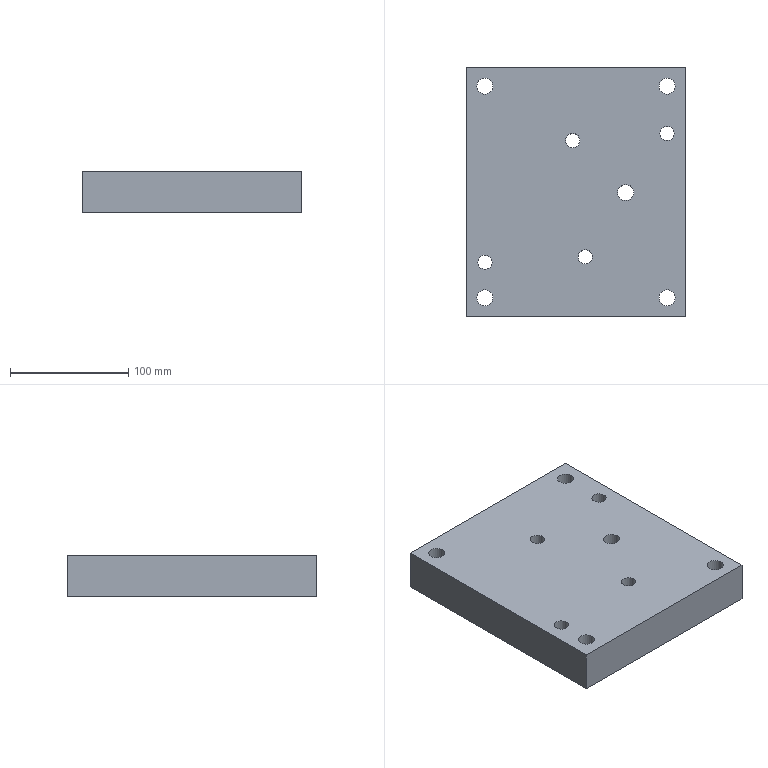Part | NX | features 7 2 | 1 solid | 37 faces | box 186 x 211 x 35 mm | volume 1310729 mm3 | cylinder 20 | plane 13 | cone 4 | commonest cylinder face diameters 13.5 x5 20 x5 10.3 x4 12.001 x4 14.11 x2
STEP:
#1=CARTESIAN_POINT('',(535.99,243.017,66.));
#2=VERTEX_POINT('',#1);
#3=CARTESIAN_POINT('',(530.84,243.017,66.));
#4=DIRECTION('',(0.,0.,1.));
#5=DIRECTION('',(1.,0.,0.));
#6=AXIS2_PLACEMENT_3D('',#3,#4,#5);
#7=CIRCLE('',#6,5.15);
#8=EDGE_CURVE('',#2,#2,#7,.T.);
#9=ORIENTED_EDGE('',*,*,#8,.T.);
#10=EDGE_LOOP('',(#9));
#11=FACE_BOUND('',#10,.T.);
#12=CARTESIAN_POINT('',(496.275,336.282,66.));
#13=VERTEX_POINT('',#12);
#14=CARTESIAN_POINT('',(490.274,336.282,66.));
#15=DIRECTION('',(0.,0.,1.));
#16=DIRECTION('',(1.,0.,0.));
#17=AXIS2_PLACEMENT_3D('',#14,#15,#16);
#18=CIRCLE('',#17,6.);
#19=EDGE_CURVE('',#13,#13,#18,.T.);
#20=ORIENTED_EDGE('',*,*,#19,.T.);
#21=EDGE_LOOP('',(#20));
#22=FACE_BOUND('',#21,.T.);
#23=CARTESIAN_POINT('',(441.424,319.282,66.));
#24=VERTEX_POINT('',#23);
#25=CARTESIAN_POINT('',(436.274,319.282,66.));
#26=DIRECTION('',(0.,0.,1.));
#27=DIRECTION('',(1.,0.,0.));
#28=AXIS2_PLACEMENT_3D('',#25,#26,#27);
#29=CIRCLE('',#28,5.15);
#30=EDGE_CURVE('',#24,#24,#29,.T.);
#31=ORIENTED_EDGE('',*,*,#30,.T.);
#32=EDGE_LOOP('',(#31));
#33=FACE_BOUND('',#32,.T.);
#34=CARTESIAN_POINT('',(577.112,342.372,66.));
#35=VERTEX_POINT('',#34);
#36=CARTESIAN_POINT('',(570.057,342.372,66.));
#37=DIRECTION('',(0.,0.,1.));
#38=DIRECTION('',(1.,0.,0.));
#39=AXIS2_PLACEMENT_3D('',#36,#37,#38);
#40=CIRCLE('',#39,7.055);
#41=EDGE_CURVE('',#35,#35,#40,.T.);
#42=ORIENTED_EDGE('',*,*,#41,.T.);
#43=EDGE_LOOP('',(#42));
#44=FACE_BOUND('',#43,.T.);
#45=CARTESIAN_POINT('',(423.112,233.372,66.));
#46=VERTEX_POINT('',#45);
#47=CARTESIAN_POINT('',(416.057,233.372,66.));
#48=DIRECTION('',(0.,0.,1.));
#49=DIRECTION('',(1.,0.,0.));
#50=AXIS2_PLACEMENT_3D('',#47,#48,#49);
#51=CIRCLE('',#50,7.055);
#52=EDGE_CURVE('',#46,#46,#51,.T.);
#53=ORIENTED_EDGE('',*,*,#52,.T.);
#54=EDGE_LOOP('',(#53));
#55=FACE_BOUND('',#54,.T.);
#56=CARTESIAN_POINT('',(525.057,292.372,66.));
#57=VERTEX_POINT('',#56);
#58=CARTESIAN_POINT('',(535.057,292.372,66.));
#59=DIRECTION('',(0.,0.,-1.));
#60=DIRECTION('',(-1.,0.,0.));
#61=AXIS2_PLACEMENT_3D('',#58,#59,#60);
#62=CIRCLE('',#61,10.);
#63=EDGE_CURVE('',#57,#57,#62,.T.);
#64=ORIENTED_EDGE('',*,*,#63,.F.);
#65=EDGE_LOOP('',(#64));
#66=FACE_BOUND('',#65,.T.);
#67=CARTESIAN_POINT('',(560.057,203.372,66.));
#68=VERTEX_POINT('',#67);
#69=CARTESIAN_POINT('',(570.057,203.372,66.));
#70=DIRECTION('',(0.,0.,1.));
#71=DIRECTION('',(-1.,0.,0.));
#72=AXIS2_PLACEMENT_3D('',#69,#70,#71);
#73=CIRCLE('',#72,10.);
#74=EDGE_CURVE('',#68,#68,#73,.T.);
#75=ORIENTED_EDGE('',*,*,#74,.T.);
#76=EDGE_LOOP('',(#75));
#77=FACE_BOUND('',#76,.T.);
#78=CARTESIAN_POINT('',(406.057,203.372,66.));
#79=VERTEX_POINT('',#78);
#80=CARTESIAN_POINT('',(416.057,203.372,66.));
#81=DIRECTION('',(0.,0.,1.));
#82=DIRECTION('',(-1.,0.,0.));
#83=AXIS2_PLACEMENT_3D('',#80,#81,#82);
#84=CIRCLE('',#83,10.);
#85=EDGE_CURVE('',#79,#79,#84,.T.);
#86=ORIENTED_EDGE('',*,*,#85,.T.);
#87=EDGE_LOOP('',(#86));
#88=FACE_BOUND('',#87,.T.);
#89=CARTESIAN_POINT('',(586.057,187.372,66.));
#90=VERTEX_POINT('',#89);
#91=CARTESIAN_POINT('',(586.057,398.372,66.));
#92=VERTEX_POINT('',#91);
#93=CARTESIAN_POINT('',(586.057,292.872,66.));
#94=DIRECTION('',(0.,1.,0.));
#95=VECTOR('',#94,1000.);
#96=LINE('',#93,#95);
#97=EDGE_CURVE('',#90,#92,#96,.T.);
#98=ORIENTED_EDGE('',*,*,#97,.F.);
#99=CARTESIAN_POINT('',(400.057,187.372,66.));
#100=VERTEX_POINT('',#99);
#101=CARTESIAN_POINT('',(493.057,187.372,66.));
#102=DIRECTION('',(1.,0.,0.));
#103=VECTOR('',#102,1000.);
#104=LINE('',#101,#103);
#105=EDGE_CURVE('',#100,#90,#104,.T.);
#106=ORIENTED_EDGE('',*,*,#105,.F.);
#107=CARTESIAN_POINT('',(400.057,398.372,66.));
#108=VERTEX_POINT('',#107);
#109=CARTESIAN_POINT('',(400.057,292.872,66.));
#110=DIRECTION('',(0.,-1.,0.));
#111=VECTOR('',#110,1000.);
#112=LINE('',#109,#111);
#113=EDGE_CURVE('',#108,#100,#112,.T.);
#114=ORIENTED_EDGE('',*,*,#113,.F.);
#115=CARTESIAN_POINT('',(493.057,398.372,66.));
#116=DIRECTION('',(-1.,0.,0.));
#117=VECTOR('',#116,1000.);
#118=LINE('',#115,#117);
#119=EDGE_CURVE('',#92,#108,#118,.T.);
#120=ORIENTED_EDGE('',*,*,#119,.F.);
#121=EDGE_LOOP('',(#98,#106,#114,#120));
#122=FACE_BOUND('',#121,.T.);
#123=CARTESIAN_POINT('',(560.057,382.372,66.));
#124=VERTEX_POINT('',#123);
#125=CARTESIAN_POINT('',(570.057,382.372,66.));
#126=DIRECTION('',(0.,0.,1.));
#127=DIRECTION('',(-1.,0.,0.));
#128=AXIS2_PLACEMENT_3D('',#125,#126,#127);
#129=CIRCLE('',#128,10.);
#130=EDGE_CURVE('',#124,#124,#129,.T.);
#131=ORIENTED_EDGE('',*,*,#130,.T.);
#132=EDGE_LOOP('',(#131));
#133=FACE_BOUND('',#132,.T.);
#134=CARTESIAN_POINT('',(406.057,382.372,66.));
#135=VERTEX_POINT('',#134);
#136=CARTESIAN_POINT('',(416.057,382.372,66.));
#137=DIRECTION('',(0.,0.,1.));
#138=DIRECTION('',(-1.,0.,0.));
#139=AXIS2_PLACEMENT_3D('',#136,#137,#138);
#140=CIRCLE('',#139,10.);
#141=EDGE_CURVE('',#135,#135,#140,.T.);
#142=ORIENTED_EDGE('',*,*,#141,.T.);
#143=EDGE_LOOP('',(#142));
#144=FACE_BOUND('',#143,.T.);
#145=CARTESIAN_POINT('',(475.99,361.282,66.));
#146=VERTEX_POINT('',#145);
#147=CARTESIAN_POINT('',(470.84,361.282,66.));
#148=DIRECTION('',(0.,0.,1.));
#149=DIRECTION('',(1.,0.,0.));
#150=AXIS2_PLACEMENT_3D('',#147,#148,#149);
#151=CIRCLE('',#150,5.15);
#152=EDGE_CURVE('',#146,#146,#151,.T.);
#153=ORIENTED_EDGE('',*,*,#152,.T.);
#154=EDGE_LOOP('',(#153));
#155=FACE_BOUND('',#154,.T.);
#156=CARTESIAN_POINT('',(506.841,238.017,66.));
#157=VERTEX_POINT('',#156);
#158=CARTESIAN_POINT('',(500.84,238.017,66.));
#159=DIRECTION('',(0.,0.,1.));
#160=DIRECTION('',(1.,0.,0.));
#161=AXIS2_PLACEMENT_3D('',#158,#159,#160);
#162=CIRCLE('',#161,6.);
#163=EDGE_CURVE('',#157,#157,#162,.T.);
#164=ORIENTED_EDGE('',*,*,#163,.T.);
#165=EDGE_LOOP('',(#164));
#166=FACE_BOUND('',#165,.T.);
#167=CARTESIAN_POINT('',(478.424,250.017,66.));
#168=VERTEX_POINT('',#167);
#169=CARTESIAN_POINT('',(473.274,250.017,66.));
#170=DIRECTION('',(0.,0.,1.));
#171=DIRECTION('',(1.,0.,0.));
#172=AXIS2_PLACEMENT_3D('',#169,#170,#171);
#173=CIRCLE('',#172,5.15);
#174=EDGE_CURVE('',#168,#168,#173,.T.);
#175=ORIENTED_EDGE('',*,*,#174,.T.);
#176=EDGE_LOOP('',(#175));
#177=FACE_BOUND('',#176,.T.);
#178=CARTESIAN_POINT('',(493.057,292.872,66.));
#179=DIRECTION('',(0.,0.,-1.));
#180=DIRECTION('',(1.,0.,0.));
#181=AXIS2_PLACEMENT_3D('',#178,#179,#180);
#182=PLANE('',#181);
#183=ADVANCED_FACE('',(#11,#22,#33,#44,#55,#66,#77,#88,#122,#133,#144,#155,#166,#177),#182,.T.);
#184=CARTESIAN_POINT('',(422.807,203.372,86.));
#185=VERTEX_POINT('',#184);
#186=CARTESIAN_POINT('',(416.057,203.372,86.));
#187=DIRECTION('',(0.,0.,1.));
#188=DIRECTION('',(1.,0.,0.));
#189=AXIS2_PLACEMENT_3D('',#186,#187,#188);
#190=CIRCLE('',#189,6.75);
#191=EDGE_CURVE('',#185,#185,#190,.T.);
#192=ORIENTED_EDGE('',*,*,#191,.T.);
#193=EDGE_LOOP('',(#192));
#194=FACE_BOUND('',#193,.T.);
#195=CARTESIAN_POINT('',(426.057,203.372,86.));
#196=VERTEX_POINT('',#195);
#197=CARTESIAN_POINT('',(416.057,203.372,86.));
#198=DIRECTION('',(0.,0.,1.));
#199=DIRECTION('',(1.,0.,0.));
#200=AXIS2_PLACEMENT_3D('',#197,#198,#199);
#201=CIRCLE('',#200,10.);
#202=EDGE_CURVE('',#196,#196,#201,.T.);
#203=ORIENTED_EDGE('',*,*,#202,.F.);
#204=EDGE_LOOP('',(#203));
#205=FACE_BOUND('',#204,.T.);
#206=CARTESIAN_POINT('',(416.057,203.372,86.));
#207=DIRECTION('',(0.,0.,1.));
#208=DIRECTION('',(-1.,0.,0.));
#209=AXIS2_PLACEMENT_3D('',#206,#207,#208);
#210=PLANE('',#209);
#211=ADVANCED_FACE('',(#194,#205),#210,.F.);
#212=CARTESIAN_POINT('',(576.807,382.372,86.));
#213=VERTEX_POINT('',#212);
#214=CARTESIAN_POINT('',(570.057,382.372,86.));
#215=DIRECTION('',(0.,0.,1.));
#216=DIRECTION('',(1.,0.,0.));
#217=AXIS2_PLACEMENT_3D('',#214,#215,#216);
#218=CIRCLE('',#217,6.75);
#219=EDGE_CURVE('',#213,#213,#218,.T.);
#220=ORIENTED_EDGE('',*,*,#219,.T.);
#221=EDGE_LOOP('',(#220));
#222=FACE_BOUND('',#221,.T.);
#223=CARTESIAN_POINT('',(580.057,382.372,86.));
#224=VERTEX_POINT('',#223);
#225=CARTESIAN_POINT('',(570.057,382.372,86.));
#226=DIRECTION('',(0.,0.,1.));
#227=DIRECTION('',(1.,0.,0.));
#228=AXIS2_PLACEMENT_3D('',#225,#226,#227);
#229=CIRCLE('',#228,10.);
#230=EDGE_CURVE('',#224,#224,#229,.T.);
#231=ORIENTED_EDGE('',*,*,#230,.F.);
#232=EDGE_LOOP('',(#231));
#233=FACE_BOUND('',#232,.T.);
#234=CARTESIAN_POINT('',(570.057,382.372,86.));
#235=DIRECTION('',(0.,0.,1.));
#236=DIRECTION('',(-1.,0.,0.));
#237=AXIS2_PLACEMENT_3D('',#234,#235,#236);
#238=PLANE('',#237);
#239=ADVANCED_FACE('',(#222,#233),#238,.F.);
#240=CARTESIAN_POINT('',(576.807,203.372,86.));
#241=VERTEX_POINT('',#240);
#242=CARTESIAN_POINT('',(570.057,203.372,86.));
#243=DIRECTION('',(0.,0.,1.));
#244=DIRECTION('',(1.,0.,0.));
#245=AXIS2_PLACEMENT_3D('',#242,#243,#244);
#246=CIRCLE('',#245,6.75);
#247=EDGE_CURVE('',#241,#241,#246,.T.);
#248=ORIENTED_EDGE('',*,*,#247,.T.);
#249=EDGE_LOOP('',(#248));
#250=FACE_BOUND('',#249,.T.);
#251=CARTESIAN_POINT('',(580.057,203.372,86.));
#252=VERTEX_POINT('',#251);
#253=CARTESIAN_POINT('',(570.057,203.372,86.));
#254=DIRECTION('',(0.,0.,1.));
#255=DIRECTION('',(1.,0.,0.));
#256=AXIS2_PLACEMENT_3D('',#253,#254,#255);
#257=CIRCLE('',#256,10.);
#258=EDGE_CURVE('',#252,#252,#257,.T.);
#259=ORIENTED_EDGE('',*,*,#258,.F.);
#260=EDGE_LOOP('',(#259));
#261=FACE_BOUND('',#260,.T.);
#262=CARTESIAN_POINT('',(570.057,203.372,86.));
#263=DIRECTION('',(0.,0.,1.));
#264=DIRECTION('',(-1.,0.,0.));
#265=AXIS2_PLACEMENT_3D('',#262,#263,#264);
#266=PLANE('',#265);
#267=ADVANCED_FACE('',(#250,#261),#266,.F.);
#268=CARTESIAN_POINT('',(422.807,382.372,86.));
#269=VERTEX_POINT('',#268);
#270=CARTESIAN_POINT('',(416.057,382.372,86.));
#271=DIRECTION('',(0.,0.,1.));
#272=DIRECTION('',(1.,0.,0.));
#273=AXIS2_PLACEMENT_3D('',#270,#271,#272);
#274=CIRCLE('',#273,6.75);
#275=EDGE_CURVE('',#269,#269,#274,.T.);
#276=ORIENTED_EDGE('',*,*,#275,.T.);
#277=EDGE_LOOP('',(#276));
#278=FACE_BOUND('',#277,.T.);
#279=CARTESIAN_POINT('',(426.057,382.372,86.));
#280=VERTEX_POINT('',#279);
#281=CARTESIAN_POINT('',(416.057,382.372,86.));
#282=DIRECTION('',(0.,0.,1.));
#283=DIRECTION('',(1.,0.,0.));
#284=AXIS2_PLACEMENT_3D('',#281,#282,#283);
#285=CIRCLE('',#284,10.);
#286=EDGE_CURVE('',#280,#280,#285,.T.);
#287=ORIENTED_EDGE('',*,*,#286,.F.);
#288=EDGE_LOOP('',(#287));
#289=FACE_BOUND('',#288,.T.);
#290=CARTESIAN_POINT('',(416.057,382.372,86.));
#291=DIRECTION('',(0.,0.,1.));
#292=DIRECTION('',(-1.,0.,0.));
#293=AXIS2_PLACEMENT_3D('',#290,#291,#292);
#294=PLANE('',#293);
#295=ADVANCED_FACE('',(#278,#289),#294,.F.);
#296=ORIENTED_EDGE('',*,*,#286,.T.);
#297=EDGE_LOOP('',(#296));
#298=FACE_BOUND('',#297,.T.);
#299=ORIENTED_EDGE('',*,*,#141,.F.);
#300=EDGE_LOOP('',(#299));
#301=FACE_BOUND('',#300,.T.);
#302=CARTESIAN_POINT('',(416.057,382.372,71.));
#303=DIRECTION('',(0.,0.,1.));
#304=DIRECTION('',(-1.,0.,0.));
#305=AXIS2_PLACEMENT_3D('',#302,#303,#304);
#306=CYLINDRICAL_SURFACE('',#305,10.);
#307=ADVANCED_FACE('',(#298,#301),#306,.F.);
#308=ORIENTED_EDGE('',*,*,#230,.T.);
#309=EDGE_LOOP('',(#308));
#310=FACE_BOUND('',#309,.T.);
#311=ORIENTED_EDGE('',*,*,#130,.F.);
#312=EDGE_LOOP('',(#311));
#313=FACE_BOUND('',#312,.T.);
#314=CARTESIAN_POINT('',(570.057,382.372,71.));
#315=DIRECTION('',(0.,0.,1.));
#316=DIRECTION('',(-1.,0.,0.));
#317=AXIS2_PLACEMENT_3D('',#314,#315,#316);
#318=CYLINDRICAL_SURFACE('',#317,10.);
#319=ADVANCED_FACE('',(#310,#313),#318,.F.);
#320=ORIENTED_EDGE('',*,*,#202,.T.);
#321=EDGE_LOOP('',(#320));
#322=FACE_BOUND('',#321,.T.);
#323=ORIENTED_EDGE('',*,*,#85,.F.);
#324=EDGE_LOOP('',(#323));
#325=FACE_BOUND('',#324,.T.);
#326=CARTESIAN_POINT('',(416.057,203.372,71.));
#327=DIRECTION('',(0.,0.,1.));
#328=DIRECTION('',(-1.,0.,0.));
#329=AXIS2_PLACEMENT_3D('',#326,#327,#328);
#330=CYLINDRICAL_SURFACE('',#329,10.);
#331=ADVANCED_FACE('',(#322,#325),#330,.F.);
#332=ORIENTED_EDGE('',*,*,#258,.T.);
#333=EDGE_LOOP('',(#332));
#334=FACE_BOUND('',#333,.T.);
#335=ORIENTED_EDGE('',*,*,#74,.F.);
#336=EDGE_LOOP('',(#335));
#337=FACE_BOUND('',#336,.T.);
#338=CARTESIAN_POINT('',(570.057,203.372,71.));
#339=DIRECTION('',(0.,0.,1.));
#340=DIRECTION('',(-1.,0.,0.));
#341=AXIS2_PLACEMENT_3D('',#338,#339,#340);
#342=CYLINDRICAL_SURFACE('',#341,10.);
#343=ADVANCED_FACE('',(#334,#337),#342,.F.);
#344=CARTESIAN_POINT('',(400.057,187.372,101.));
#345=VERTEX_POINT('',#344);
#346=CARTESIAN_POINT('',(400.057,187.372,71.));
#347=DIRECTION('',(0.,0.,1.));
#348=VECTOR('',#347,1000.);
#349=LINE('',#346,#348);
#350=EDGE_CURVE('',#100,#345,#349,.T.);
#351=ORIENTED_EDGE('',*,*,#350,.T.);
#352=CARTESIAN_POINT('',(400.057,398.372,101.));
#353=VERTEX_POINT('',#352);
#354=CARTESIAN_POINT('',(400.057,292.872,101.));
#355=DIRECTION('',(0.,1.,0.));
#356=VECTOR('',#355,1000.);
#357=LINE('',#354,#356);
#358=EDGE_CURVE('',#345,#353,#357,.T.);
#359=ORIENTED_EDGE('',*,*,#358,.T.);
#360=CARTESIAN_POINT('',(400.057,398.372,71.));
#361=DIRECTION('',(0.,0.,1.));
#362=VECTOR('',#361,1000.);
#363=LINE('',#360,#362);
#364=EDGE_CURVE('',#108,#353,#363,.T.);
#365=ORIENTED_EDGE('',*,*,#364,.F.);
#366=ORIENTED_EDGE('',*,*,#113,.T.);
#367=EDGE_LOOP('',(#351,#359,#365,#366));
#368=FACE_BOUND('',#367,.T.);
#369=CARTESIAN_POINT('',(400.057,292.872,71.));
#370=DIRECTION('',(-1.,0.,0.));
#371=DIRECTION('',(0.,0.,-1.));
#372=AXIS2_PLACEMENT_3D('',#369,#370,#371);
#373=PLANE('',#372);
#374=ADVANCED_FACE('',(#368),#373,.T.);
#375=ORIENTED_EDGE('',*,*,#364,.T.);
#376=CARTESIAN_POINT('',(586.057,398.372,101.));
#377=VERTEX_POINT('',#376);
#378=CARTESIAN_POINT('',(493.057,398.372,101.));
#379=DIRECTION('',(1.,0.,0.));
#380=VECTOR('',#379,1000.);
#381=LINE('',#378,#380);
#382=EDGE_CURVE('',#353,#377,#381,.T.);
#383=ORIENTED_EDGE('',*,*,#382,.T.);
#384=CARTESIAN_POINT('',(586.057,398.372,71.));
#385=DIRECTION('',(0.,0.,1.));
#386=VECTOR('',#385,1000.);
#387=LINE('',#384,#386);
#388=EDGE_CURVE('',#92,#377,#387,.T.);
#389=ORIENTED_EDGE('',*,*,#388,.F.);
#390=ORIENTED_EDGE('',*,*,#119,.T.);
#391=EDGE_LOOP('',(#375,#383,#389,#390));
#392=FACE_BOUND('',#391,.T.);
#393=CARTESIAN_POINT('',(493.057,398.372,71.));
#394=DIRECTION('',(0.,1.,0.));
#395=DIRECTION('',(0.,0.,-1.));
#396=AXIS2_PLACEMENT_3D('',#393,#394,#395);
#397=PLANE('',#396);
#398=ADVANCED_FACE('',(#392),#397,.T.);
#399=ORIENTED_EDGE('',*,*,#97,.T.);
#400=ORIENTED_EDGE('',*,*,#388,.T.);
#401=CARTESIAN_POINT('',(586.057,187.372,101.));
#402=VERTEX_POINT('',#401);
#403=CARTESIAN_POINT('',(586.057,292.872,101.));
#404=DIRECTION('',(0.,-1.,0.));
#405=VECTOR('',#404,1000.);
#406=LINE('',#403,#405);
#407=EDGE_CURVE('',#377,#402,#406,.T.);
#408=ORIENTED_EDGE('',*,*,#407,.T.);
#409=CARTESIAN_POINT('',(586.057,187.372,71.));
#410=DIRECTION('',(0.,0.,1.));
#411=VECTOR('',#410,1000.);
#412=LINE('',#409,#411);
#413=EDGE_CURVE('',#90,#402,#412,.T.);
#414=ORIENTED_EDGE('',*,*,#413,.F.);
#415=EDGE_LOOP('',(#399,#400,#408,#414));
#416=FACE_BOUND('',#415,.T.);
#417=CARTESIAN_POINT('',(586.057,292.872,71.));
#418=DIRECTION('',(1.,0.,0.));
#419=DIRECTION('',(0.,0.,1.));
#420=AXIS2_PLACEMENT_3D('',#417,#418,#419);
#421=PLANE('',#420);
#422=ADVANCED_FACE('',(#416),#421,.T.);
#423=ORIENTED_EDGE('',*,*,#413,.T.);
#424=CARTESIAN_POINT('',(493.057,187.372,101.));
#425=DIRECTION('',(-1.,0.,0.));
#426=VECTOR('',#425,1000.);
#427=LINE('',#424,#426);
#428=EDGE_CURVE('',#402,#345,#427,.T.);
#429=ORIENTED_EDGE('',*,*,#428,.T.);
#430=ORIENTED_EDGE('',*,*,#350,.F.);
#431=ORIENTED_EDGE('',*,*,#105,.T.);
#432=EDGE_LOOP('',(#423,#429,#430,#431));
#433=FACE_BOUND('',#432,.T.);
#434=CARTESIAN_POINT('',(493.057,187.372,71.));
#435=DIRECTION('',(0.,-1.,0.));
#436=DIRECTION('',(0.,0.,1.));
#437=AXIS2_PLACEMENT_3D('',#434,#435,#436);
#438=PLANE('',#437);
#439=ADVANCED_FACE('',(#433),#438,.T.);
#440=CARTESIAN_POINT('',(422.807,203.372,101.));
#441=VERTEX_POINT('',#440);
#442=CARTESIAN_POINT('',(416.057,203.372,101.));
#443=DIRECTION('',(0.,0.,1.));
#444=DIRECTION('',(1.,0.,0.));
#445=AXIS2_PLACEMENT_3D('',#442,#443,#444);
#446=CIRCLE('',#445,6.75);
#447=EDGE_CURVE('',#441,#441,#446,.T.);
#448=ORIENTED_EDGE('',*,*,#447,.T.);
#449=EDGE_LOOP('',(#448));
#450=FACE_BOUND('',#449,.T.);
#451=ORIENTED_EDGE('',*,*,#191,.F.);
#452=EDGE_LOOP('',(#451));
#453=FACE_BOUND('',#452,.T.);
#454=CARTESIAN_POINT('',(416.057,203.372,68.));
#455=DIRECTION('',(0.,0.,1.));
#456=DIRECTION('',(-1.,0.,0.));
#457=AXIS2_PLACEMENT_3D('',#454,#455,#456);
#458=CYLINDRICAL_SURFACE('',#457,6.75);
#459=ADVANCED_FACE('',(#450,#453),#458,.F.);
#460=CARTESIAN_POINT('',(576.807,382.372,101.));
#461=VERTEX_POINT('',#460);
#462=CARTESIAN_POINT('',(570.057,382.372,101.));
#463=DIRECTION('',(0.,0.,1.));
#464=DIRECTION('',(1.,0.,0.));
#465=AXIS2_PLACEMENT_3D('',#462,#463,#464);
#466=CIRCLE('',#465,6.75);
#467=EDGE_CURVE('',#461,#461,#466,.T.);
#468=ORIENTED_EDGE('',*,*,#467,.T.);
#469=EDGE_LOOP('',(#468));
#470=FACE_BOUND('',#469,.T.);
#471=ORIENTED_EDGE('',*,*,#219,.F.);
#472=EDGE_LOOP('',(#471));
#473=FACE_BOUND('',#472,.T.);
#474=CARTESIAN_POINT('',(570.057,382.372,68.));
#475=DIRECTION('',(0.,0.,1.));
#476=DIRECTION('',(-1.,0.,0.));
#477=AXIS2_PLACEMENT_3D('',#474,#475,#476);
#478=CYLINDRICAL_SURFACE('',#477,6.75);
#479=ADVANCED_FACE('',(#470,#473),#478,.F.);
#480=CARTESIAN_POINT('',(576.807,203.372,101.));
#481=VERTEX_POINT('',#480);
#482=CARTESIAN_POINT('',(570.057,203.372,101.));
#483=DIRECTION('',(0.,0.,1.));
#484=DIRECTION('',(1.,0.,0.));
#485=AXIS2_PLACEMENT_3D('',#482,#483,#484);
#486=CIRCLE('',#485,6.75);
#487=EDGE_CURVE('',#481,#481,#486,.T.);
#488=ORIENTED_EDGE('',*,*,#487,.T.);
#489=EDGE_LOOP('',(#488));
#490=FACE_BOUND('',#489,.T.);
#491=ORIENTED_EDGE('',*,*,#247,.F.);
#492=EDGE_LOOP('',(#491));
#493=FACE_BOUND('',#492,.T.);
#494=CARTESIAN_POINT('',(570.057,203.372,68.));
#495=DIRECTION('',(0.,0.,1.));
#496=DIRECTION('',(-1.,0.,0.));
#497=AXIS2_PLACEMENT_3D('',#494,#495,#496);
#498=CYLINDRICAL_SURFACE('',#497,6.75);
#499=ADVANCED_FACE('',(#490,#493),#498,.F.);
#500=CARTESIAN_POINT('',(422.807,382.372,101.));
#501=VERTEX_POINT('',#500);
#502=CARTESIAN_POINT('',(416.057,382.372,101.));
#503=DIRECTION('',(0.,0.,1.));
#504=DIRECTION('',(1.,0.,0.));
#505=AXIS2_PLACEMENT_3D('',#502,#503,#504);
#506=CIRCLE('',#505,6.75);
#507=EDGE_CURVE('',#501,#501,#506,.T.);
#508=ORIENTED_EDGE('',*,*,#507,.T.);
#509=EDGE_LOOP('',(#508));
#510=FACE_BOUND('',#509,.T.);
#511=ORIENTED_EDGE('',*,*,#275,.F.);
#512=EDGE_LOOP('',(#511));
#513=FACE_BOUND('',#512,.T.);
#514=CARTESIAN_POINT('',(416.057,382.372,68.));
#515=DIRECTION('',(0.,0.,1.));
#516=DIRECTION('',(-1.,0.,0.));
#517=AXIS2_PLACEMENT_3D('',#514,#515,#516);
#518=CYLINDRICAL_SURFACE('',#517,6.75);
#519=ADVANCED_FACE('',(#510,#513),#518,.F.);
#520=CARTESIAN_POINT('',(422.058,233.372,78.));
#521=VERTEX_POINT('',#520);
#522=CARTESIAN_POINT('',(416.057,233.372,78.));
#523=DIRECTION('',(0.,0.,-1.));
#524=DIRECTION('',(1.,0.,0.));
#525=AXIS2_PLACEMENT_3D('',#522,#523,#524);
#526=CIRCLE('',#525,6.);
#527=EDGE_CURVE('',#521,#521,#526,.T.);
#528=ORIENTED_EDGE('',*,*,#527,.T.);
#529=EDGE_LOOP('',(#528));
#530=FACE_BOUND('',#529,.T.);
#531=CARTESIAN_POINT('',(422.058,233.372,101.));
#532=VERTEX_POINT('',#531);
#533=CARTESIAN_POINT('',(416.057,233.372,101.));
#534=DIRECTION('',(0.,0.,1.));
#535=DIRECTION('',(1.,0.,0.));
#536=AXIS2_PLACEMENT_3D('',#533,#534,#535);
#537=CIRCLE('',#536,6.);
#538=EDGE_CURVE('',#532,#532,#537,.T.);
#539=ORIENTED_EDGE('',*,*,#538,.T.);
#540=EDGE_LOOP('',(#539));
#541=FACE_BOUND('',#540,.T.);
#542=CARTESIAN_POINT('',(416.057,233.372,68.));
#543=DIRECTION('',(0.,0.,1.));
#544=DIRECTION('',(-1.,0.,0.));
#545=AXIS2_PLACEMENT_3D('',#542,#543,#544);
#546=CYLINDRICAL_SURFACE('',#545,6.);
#547=ADVANCED_FACE('',(#530,#541),#546,.F.);
#548=CARTESIAN_POINT('',(576.058,342.372,78.));
#549=VERTEX_POINT('',#548);
#550=CARTESIAN_POINT('',(570.057,342.372,78.));
#551=DIRECTION('',(0.,0.,-1.));
#552=DIRECTION('',(1.,0.,0.));
#553=AXIS2_PLACEMENT_3D('',#550,#551,#552);
#554=CIRCLE('',#553,6.);
#555=EDGE_CURVE('',#549,#549,#554,.T.);
#556=ORIENTED_EDGE('',*,*,#555,.T.);
#557=EDGE_LOOP('',(#556));
#558=FACE_BOUND('',#557,.T.);
#559=CARTESIAN_POINT('',(576.058,342.372,101.));
#560=VERTEX_POINT('',#559);
#561=CARTESIAN_POINT('',(570.057,342.372,101.));
#562=DIRECTION('',(0.,0.,1.));
#563=DIRECTION('',(1.,0.,0.));
#564=AXIS2_PLACEMENT_3D('',#561,#562,#563);
#565=CIRCLE('',#564,6.);
#566=EDGE_CURVE('',#560,#560,#565,.T.);
#567=ORIENTED_EDGE('',*,*,#566,.T.);
#568=EDGE_LOOP('',(#567));
#569=FACE_BOUND('',#568,.T.);
#570=CARTESIAN_POINT('',(570.057,342.372,68.));
#571=DIRECTION('',(0.,0.,1.));
#572=DIRECTION('',(-1.,0.,0.));
#573=AXIS2_PLACEMENT_3D('',#570,#571,#572);
#574=CYLINDRICAL_SURFACE('',#573,6.);
#575=ADVANCED_FACE('',(#558,#569),#574,.F.);
#576=CARTESIAN_POINT('',(506.841,238.017,101.));
#577=VERTEX_POINT('',#576);
#578=CARTESIAN_POINT('',(500.84,238.017,101.));
#579=DIRECTION('',(0.,0.,1.));
#580=DIRECTION('',(1.,0.,0.));
#581=AXIS2_PLACEMENT_3D('',#578,#579,#580);
#582=CIRCLE('',#581,6.);
#583=EDGE_CURVE('',#577,#577,#582,.T.);
#584=ORIENTED_EDGE('',*,*,#583,.F.);
#585=EDGE_LOOP('',(#584));
#586=FACE_BOUND('',#585,.T.);
#587=CARTESIAN_POINT('',(496.275,336.282,101.));
#588=VERTEX_POINT('',#587);
#589=CARTESIAN_POINT('',(490.274,336.282,101.));
#590=DIRECTION('',(0.,0.,1.));
#591=DIRECTION('',(1.,0.,0.));
#592=AXIS2_PLACEMENT_3D('',#589,#590,#591);
#593=CIRCLE('',#592,6.);
#594=EDGE_CURVE('',#588,#588,#593,.T.);
#595=ORIENTED_EDGE('',*,*,#594,.F.);
#596=EDGE_LOOP('',(#595));
#597=FACE_BOUND('',#596,.T.);
#598=CARTESIAN_POINT('',(541.807,292.372,101.));
#599=VERTEX_POINT('',#598);
#600=CARTESIAN_POINT('',(535.057,292.372,101.));
#601=DIRECTION('',(0.,0.,1.));
#602=DIRECTION('',(1.,0.,0.));
#603=AXIS2_PLACEMENT_3D('',#600,#601,#602);
#604=CIRCLE('',#603,6.75);
#605=EDGE_CURVE('',#599,#599,#604,.T.);
#606=ORIENTED_EDGE('',*,*,#605,.F.);
#607=EDGE_LOOP('',(#606));
#608=FACE_BOUND('',#607,.T.);
#609=ORIENTED_EDGE('',*,*,#566,.F.);
#610=EDGE_LOOP('',(#609));
#611=FACE_BOUND('',#610,.T.);
#612=ORIENTED_EDGE('',*,*,#538,.F.);
#613=EDGE_LOOP('',(#612));
#614=FACE_BOUND('',#613,.T.);
#615=ORIENTED_EDGE('',*,*,#507,.F.);
#616=EDGE_LOOP('',(#615));
#617=FACE_BOUND('',#616,.T.);
#618=ORIENTED_EDGE('',*,*,#487,.F.);
#619=EDGE_LOOP('',(#618));
#620=FACE_BOUND('',#619,.T.);
#621=ORIENTED_EDGE('',*,*,#467,.F.);
#622=EDGE_LOOP('',(#621));
#623=FACE_BOUND('',#622,.T.);
#624=ORIENTED_EDGE('',*,*,#447,.F.);
#625=EDGE_LOOP('',(#624));
#626=FACE_BOUND('',#625,.T.);
#627=ORIENTED_EDGE('',*,*,#428,.F.);
#628=ORIENTED_EDGE('',*,*,#407,.F.);
#629=ORIENTED_EDGE('',*,*,#382,.F.);
#630=ORIENTED_EDGE('',*,*,#358,.F.);
#631=EDGE_LOOP('',(#627,#628,#629,#630));
#632=FACE_BOUND('',#631,.T.);
#633=CARTESIAN_POINT('',(493.057,292.872,101.));
#634=DIRECTION('',(0.,0.,1.));
#635=DIRECTION('',(-1.,0.,0.));
#636=AXIS2_PLACEMENT_3D('',#633,#634,#635);
#637=PLANE('',#636);
#638=ADVANCED_FACE('',(#586,#597,#608,#611,#614,#617,#620,#623,#626,#632),#637,.T.);
#639=CARTESIAN_POINT('',(541.807,292.372,86.));
#640=VERTEX_POINT('',#639);
#641=CARTESIAN_POINT('',(535.057,292.372,86.));
#642=DIRECTION('',(0.,0.,1.));
#643=DIRECTION('',(1.,0.,0.));
#644=AXIS2_PLACEMENT_3D('',#641,#642,#643);
#645=CIRCLE('',#644,6.75);
#646=EDGE_CURVE('',#640,#640,#645,.T.);
#647=ORIENTED_EDGE('',*,*,#646,.T.);
#648=EDGE_LOOP('',(#647));
#649=FACE_BOUND('',#648,.T.);
#650=CARTESIAN_POINT('',(545.057,292.372,86.));
#651=VERTEX_POINT('',#650);
#652=CARTESIAN_POINT('',(535.057,292.372,86.));
#653=DIRECTION('',(0.,0.,1.));
#654=DIRECTION('',(1.,0.,0.));
#655=AXIS2_PLACEMENT_3D('',#652,#653,#654);
#656=CIRCLE('',#655,10.);
#657=EDGE_CURVE('',#651,#651,#656,.T.);
#658=ORIENTED_EDGE('',*,*,#657,.F.);
#659=EDGE_LOOP('',(#658));
#660=FACE_BOUND('',#659,.T.);
#661=CARTESIAN_POINT('',(535.057,292.372,86.));
#662=DIRECTION('',(0.,0.,1.));
#663=DIRECTION('',(-1.,0.,0.));
#664=AXIS2_PLACEMENT_3D('',#661,#662,#663);
#665=PLANE('',#664);
#666=ADVANCED_FACE('',(#649,#660),#665,.F.);
#667=ORIENTED_EDGE('',*,*,#605,.T.);
#668=EDGE_LOOP('',(#667));
#669=FACE_BOUND('',#668,.T.);
#670=ORIENTED_EDGE('',*,*,#646,.F.);
#671=EDGE_LOOP('',(#670));
#672=FACE_BOUND('',#671,.T.);
#673=CARTESIAN_POINT('',(535.057,292.372,68.));
#674=DIRECTION('',(0.,0.,1.));
#675=DIRECTION('',(-1.,0.,0.));
#676=AXIS2_PLACEMENT_3D('',#673,#674,#675);
#677=CYLINDRICAL_SURFACE('',#676,6.75);
#678=ADVANCED_FACE('',(#669,#672),#677,.F.);
#679=ORIENTED_EDGE('',*,*,#657,.T.);
#680=EDGE_LOOP('',(#679));
#681=FACE_BOUND('',#680,.T.);
#682=ORIENTED_EDGE('',*,*,#63,.T.);
#683=EDGE_LOOP('',(#682));
#684=FACE_BOUND('',#683,.T.);
#685=CARTESIAN_POINT('',(535.057,292.372,71.));
#686=DIRECTION('',(0.,0.,1.));
#687=DIRECTION('',(-1.,0.,0.));
#688=AXIS2_PLACEMENT_3D('',#685,#686,#687);
#689=CYLINDRICAL_SURFACE('',#688,10.);
#690=ADVANCED_FACE('',(#681,#684),#689,.F.);
#691=CARTESIAN_POINT('',(423.112,233.372,78.));
#692=VERTEX_POINT('',#691);
#693=CARTESIAN_POINT('',(416.057,233.372,78.));
#694=DIRECTION('',(0.,0.,-1.));
#695=DIRECTION('',(1.,0.,0.));
#696=AXIS2_PLACEMENT_3D('',#693,#694,#695);
#697=CIRCLE('',#696,7.055);
#698=EDGE_CURVE('',#692,#692,#697,.T.);
#699=ORIENTED_EDGE('',*,*,#698,.T.);
#700=EDGE_LOOP('',(#699));
#701=FACE_BOUND('',#700,.T.);
#702=ORIENTED_EDGE('',*,*,#527,.F.);
#703=EDGE_LOOP('',(#702));
#704=FACE_BOUND('',#703,.T.);
#705=CARTESIAN_POINT('',(416.057,233.372,78.));
#706=DIRECTION('',(0.,0.,1.));
#707=DIRECTION('',(-1.,0.,0.));
#708=AXIS2_PLACEMENT_3D('',#705,#706,#707);
#709=PLANE('',#708);
#710=ADVANCED_FACE('',(#701,#704),#709,.F.);
#711=ORIENTED_EDGE('',*,*,#698,.F.);
#712=EDGE_LOOP('',(#711));
#713=FACE_BOUND('',#712,.T.);
#714=ORIENTED_EDGE('',*,*,#52,.F.);
#715=EDGE_LOOP('',(#714));
#716=FACE_BOUND('',#715,.T.);
#717=CARTESIAN_POINT('',(416.057,233.372,66.));
#718=DIRECTION('',(0.,0.,1.));
#719=DIRECTION('',(-1.,0.,0.));
#720=AXIS2_PLACEMENT_3D('',#717,#718,#719);
#721=CYLINDRICAL_SURFACE('',#720,7.055);
#722=ADVANCED_FACE('',(#713,#716),#721,.F.);
#723=CARTESIAN_POINT('',(577.112,342.372,78.));
#724=VERTEX_POINT('',#723);
#725=CARTESIAN_POINT('',(570.057,342.372,78.));
#726=DIRECTION('',(0.,0.,-1.));
#727=DIRECTION('',(1.,0.,0.));
#728=AXIS2_PLACEMENT_3D('',#725,#726,#727);
#729=CIRCLE('',#728,7.055);
#730=EDGE_CURVE('',#724,#724,#729,.T.);
#731=ORIENTED_EDGE('',*,*,#730,.T.);
#732=EDGE_LOOP('',(#731));
#733=FACE_BOUND('',#732,.T.);
#734=ORIENTED_EDGE('',*,*,#555,.F.);
#735=EDGE_LOOP('',(#734));
#736=FACE_BOUND('',#735,.T.);
#737=CARTESIAN_POINT('',(570.057,342.372,78.));
#738=DIRECTION('',(0.,0.,1.));
#739=DIRECTION('',(-1.,0.,0.));
#740=AXIS2_PLACEMENT_3D('',#737,#738,#739);
#741=PLANE('',#740);
#742=ADVANCED_FACE('',(#733,#736),#741,.F.);
#743=ORIENTED_EDGE('',*,*,#730,.F.);
#744=EDGE_LOOP('',(#743));
#745=FACE_BOUND('',#744,.T.);
#746=ORIENTED_EDGE('',*,*,#41,.F.);
#747=EDGE_LOOP('',(#746));
#748=FACE_BOUND('',#747,.T.);
#749=CARTESIAN_POINT('',(570.057,342.372,66.));
#750=DIRECTION('',(0.,0.,1.));
#751=DIRECTION('',(-1.,0.,0.));
#752=AXIS2_PLACEMENT_3D('',#749,#750,#751);
#753=CYLINDRICAL_SURFACE('',#752,7.055);
#754=ADVANCED_FACE('',(#745,#748),#753,.F.);
#755=CARTESIAN_POINT('',(441.424,319.282,75.85));
#756=VERTEX_POINT('',#755);
#757=CARTESIAN_POINT('',(436.274,319.282,75.85));
#758=DIRECTION('',(0.,0.,1.));
#759=DIRECTION('',(1.,0.,0.));
#760=AXIS2_PLACEMENT_3D('',#757,#758,#759);
#761=CIRCLE('',#760,5.15);
#762=EDGE_CURVE('',#756,#756,#761,.T.);
#763=ORIENTED_EDGE('',*,*,#762,.T.);
#764=EDGE_LOOP('',(#763));
#765=FACE_BOUND('',#764,.T.);
#766=ORIENTED_EDGE('',*,*,#30,.F.);
#767=EDGE_LOOP('',(#766));
#768=FACE_BOUND('',#767,.T.);
#769=CARTESIAN_POINT('',(436.274,319.282,66.));
#770=DIRECTION('',(0.,0.,1.));
#771=DIRECTION('',(-1.,0.,0.));
#772=AXIS2_PLACEMENT_3D('',#769,#770,#771);
#773=CYLINDRICAL_SURFACE('',#772,5.15);
#774=ADVANCED_FACE('',(#765,#768),#773,.F.);
#775=CARTESIAN_POINT('',(436.274,319.282,81.));
#776=VERTEX_POINT('',#775);
#777=VERTEX_LOOP('',#776);
#778=FACE_BOUND('',#777,.T.);
#779=ORIENTED_EDGE('',*,*,#762,.F.);
#780=EDGE_LOOP('',(#779));
#781=FACE_BOUND('',#780,.T.);
#782=CARTESIAN_POINT('',(436.274,319.282,75.85));
#783=DIRECTION('',(0.,0.,-1.));
#784=DIRECTION('',(1.,0.,0.));
#785=AXIS2_PLACEMENT_3D('',#782,#783,#784);
#786=CONICAL_SURFACE('',#785,5.15,0.7854);
#787=ADVANCED_FACE('',(#778,#781),#786,.F.);
#788=CARTESIAN_POINT('',(475.99,361.282,75.85));
#789=VERTEX_POINT('',#788);
#790=CARTESIAN_POINT('',(470.84,361.282,75.85));
#791=DIRECTION('',(0.,0.,1.));
#792=DIRECTION('',(1.,0.,0.));
#793=AXIS2_PLACEMENT_3D('',#790,#791,#792);
#794=CIRCLE('',#793,5.15);
#795=EDGE_CURVE('',#789,#789,#794,.T.);
#796=ORIENTED_EDGE('',*,*,#795,.T.);
#797=EDGE_LOOP('',(#796));
#798=FACE_BOUND('',#797,.T.);
#799=ORIENTED_EDGE('',*,*,#152,.F.);
#800=EDGE_LOOP('',(#799));
#801=FACE_BOUND('',#800,.T.);
#802=CARTESIAN_POINT('',(470.84,361.282,66.));
#803=DIRECTION('',(0.,0.,1.));
#804=DIRECTION('',(-1.,0.,0.));
#805=AXIS2_PLACEMENT_3D('',#802,#803,#804);
#806=CYLINDRICAL_SURFACE('',#805,5.15);
#807=ADVANCED_FACE('',(#798,#801),#806,.F.);
#808=CARTESIAN_POINT('',(470.84,361.282,81.));
#809=VERTEX_POINT('',#808);
#810=VERTEX_LOOP('',#809);
#811=FACE_BOUND('',#810,.T.);
#812=ORIENTED_EDGE('',*,*,#795,.F.);
#813=EDGE_LOOP('',(#812));
#814=FACE_BOUND('',#813,.T.);
#815=CARTESIAN_POINT('',(470.84,361.282,75.85));
#816=DIRECTION('',(0.,0.,-1.));
#817=DIRECTION('',(1.,0.,0.));
#818=AXIS2_PLACEMENT_3D('',#815,#816,#817);
#819=CONICAL_SURFACE('',#818,5.15,0.7854);
#820=ADVANCED_FACE('',(#811,#814),#819,.F.);
#821=ORIENTED_EDGE('',*,*,#594,.T.);
#822=EDGE_LOOP('',(#821));
#823=FACE_BOUND('',#822,.T.);
#824=ORIENTED_EDGE('',*,*,#19,.F.);
#825=EDGE_LOOP('',(#824));
#826=FACE_BOUND('',#825,.T.);
#827=CARTESIAN_POINT('',(490.274,336.282,66.));
#828=DIRECTION('',(0.,0.,1.));
#829=DIRECTION('',(-1.,0.,0.));
#830=AXIS2_PLACEMENT_3D('',#827,#828,#829);
#831=CYLINDRICAL_SURFACE('',#830,6.);
#832=ADVANCED_FACE('',(#823,#826),#831,.F.);
#833=ORIENTED_EDGE('',*,*,#583,.T.);
#834=EDGE_LOOP('',(#833));
#835=FACE_BOUND('',#834,.T.);
#836=ORIENTED_EDGE('',*,*,#163,.F.);
#837=EDGE_LOOP('',(#836));
#838=FACE_BOUND('',#837,.T.);
#839=CARTESIAN_POINT('',(500.84,238.017,66.));
#840=DIRECTION('',(0.,0.,1.));
#841=DIRECTION('',(-1.,0.,0.));
#842=AXIS2_PLACEMENT_3D('',#839,#840,#841);
#843=CYLINDRICAL_SURFACE('',#842,6.);
#844=ADVANCED_FACE('',(#835,#838),#843,.F.);
#845=CARTESIAN_POINT('',(535.99,243.017,75.85));
#846=VERTEX_POINT('',#845);
#847=CARTESIAN_POINT('',(530.84,243.017,75.85));
#848=DIRECTION('',(0.,0.,1.));
#849=DIRECTION('',(1.,0.,0.));
#850=AXIS2_PLACEMENT_3D('',#847,#848,#849);
#851=CIRCLE('',#850,5.15);
#852=EDGE_CURVE('',#846,#846,#851,.T.);
#853=ORIENTED_EDGE('',*,*,#852,.T.);
#854=EDGE_LOOP('',(#853));
#855=FACE_BOUND('',#854,.T.);
#856=ORIENTED_EDGE('',*,*,#8,.F.);
#857=EDGE_LOOP('',(#856));
#858=FACE_BOUND('',#857,.T.);
#859=CARTESIAN_POINT('',(530.84,243.017,66.));
#860=DIRECTION('',(0.,0.,1.));
#861=DIRECTION('',(-1.,0.,0.));
#862=AXIS2_PLACEMENT_3D('',#859,#860,#861);
#863=CYLINDRICAL_SURFACE('',#862,5.15);
#864=ADVANCED_FACE('',(#855,#858),#863,.F.);
#865=CARTESIAN_POINT('',(530.84,243.017,81.));
#866=VERTEX_POINT('',#865);
#867=VERTEX_LOOP('',#866);
#868=FACE_BOUND('',#867,.T.);
#869=ORIENTED_EDGE('',*,*,#852,.F.);
#870=EDGE_LOOP('',(#869));
#871=FACE_BOUND('',#870,.T.);
#872=CARTESIAN_POINT('',(530.84,243.017,75.85));
#873=DIRECTION('',(0.,0.,-1.));
#874=DIRECTION('',(1.,0.,0.));
#875=AXIS2_PLACEMENT_3D('',#872,#873,#874);
#876=CONICAL_SURFACE('',#875,5.15,0.7854);
#877=ADVANCED_FACE('',(#868,#871),#876,.F.);
#878=CARTESIAN_POINT('',(478.424,250.017,75.85));
#879=VERTEX_POINT('',#878);
#880=CARTESIAN_POINT('',(473.274,250.017,75.85));
#881=DIRECTION('',(0.,0.,1.));
#882=DIRECTION('',(1.,0.,0.));
#883=AXIS2_PLACEMENT_3D('',#880,#881,#882);
#884=CIRCLE('',#883,5.15);
#885=EDGE_CURVE('',#879,#879,#884,.T.);
#886=ORIENTED_EDGE('',*,*,#885,.T.);
#887=EDGE_LOOP('',(#886));
#888=FACE_BOUND('',#887,.T.);
#889=ORIENTED_EDGE('',*,*,#174,.F.);
#890=EDGE_LOOP('',(#889));
#891=FACE_BOUND('',#890,.T.);
#892=CARTESIAN_POINT('',(473.274,250.017,66.));
#893=DIRECTION('',(0.,0.,1.));
#894=DIRECTION('',(-1.,0.,0.));
#895=AXIS2_PLACEMENT_3D('',#892,#893,#894);
#896=CYLINDRICAL_SURFACE('',#895,5.15);
#897=ADVANCED_FACE('',(#888,#891),#896,.F.);
#898=CARTESIAN_POINT('',(473.274,250.017,81.));
#899=VERTEX_POINT('',#898);
#900=VERTEX_LOOP('',#899);
#901=FACE_BOUND('',#900,.T.);
#902=ORIENTED_EDGE('',*,*,#885,.F.);
#903=EDGE_LOOP('',(#902));
#904=FACE_BOUND('',#903,.T.);
#905=CARTESIAN_POINT('',(473.274,250.017,75.85));
#906=DIRECTION('',(0.,0.,-1.));
#907=DIRECTION('',(1.,0.,0.));
#908=AXIS2_PLACEMENT_3D('',#905,#906,#907);
#909=CONICAL_SURFACE('',#908,5.15,0.7854);
#910=ADVANCED_FACE('',(#901,#904),#909,.F.);
#911=CLOSED_SHELL('',(#183,#211,#239,#267,#295,#307,#319,#331,#343,#374,#398,#422,#439,#459,#479,#499,#519,#547,#575,#638,#666,#678,#690,#710,#722,#742,#754,#774,#787,#807,#820,#832,#844,#864,#877,#897,#910));
#912=MANIFOLD_SOLID_BREP('',#911);
#913=(LENGTH_UNIT()NAMED_UNIT(*)SI_UNIT(.MILLI.,.METRE.));
#914=UNCERTAINTY_MEASURE_WITH_UNIT(LENGTH_MEASURE(0.00001),#913,'','');
#915=(NAMED_UNIT(*)PLANE_ANGLE_UNIT()SI_UNIT($,.RADIAN.));
#916=(NAMED_UNIT(*)SI_UNIT($,.STERADIAN.)SOLID_ANGLE_UNIT());
#917=(GEOMETRIC_REPRESENTATION_CONTEXT(3)GLOBAL_UNCERTAINTY_ASSIGNED_CONTEXT((#914))GLOBAL_UNIT_ASSIGNED_CONTEXT((#913,#915,#916))REPRESENTATION_CONTEXT('',''));
#918=ADVANCED_BREP_SHAPE_REPRESENTATION('',(#912),#917);